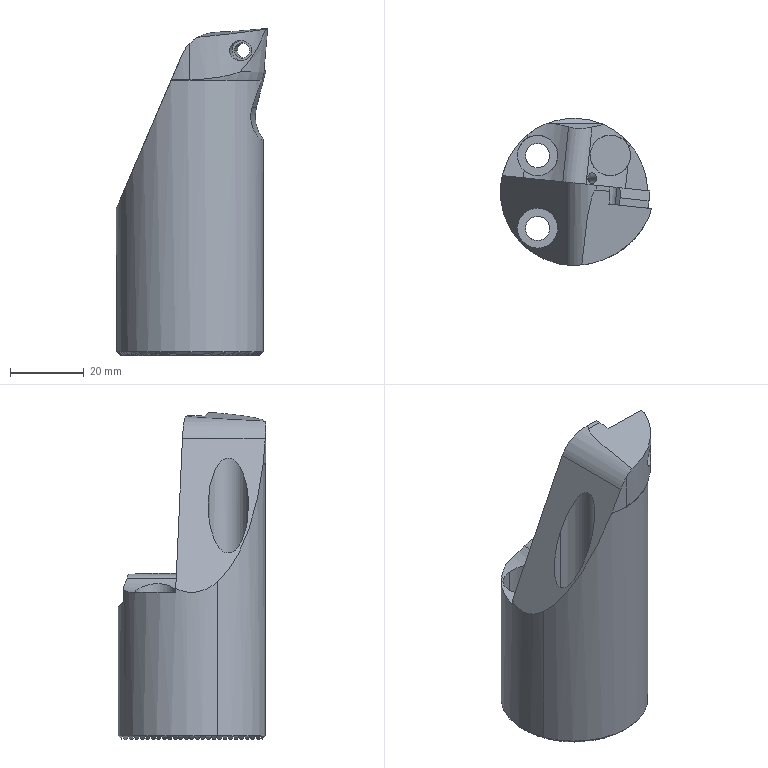NC program | Mastercam | posted with a generic post
Lines 3202 to 3213 of 11394:
(3 DR |TOOL - 3|DIA. OFF. - 3|LEN. - 3|TOOL DIA. - 3.)
N6466 T3 M6
N6468 G0 G55 G90 X10.017 Y-3.7 C90. B-20. S2000 M3
N6470 G43 H3 Z93.314
N6472 G81 G98 Z32.814 R44.314 F20.
N6474 G80
N6476 M5
N6478 G0 G28 G91 Z0.
N6480 G28 C0. B0.
N6482 M01
N6484 G0 G17 G40 G80 G90 G94 G98
N6486 G0 G28 G91 Z0.